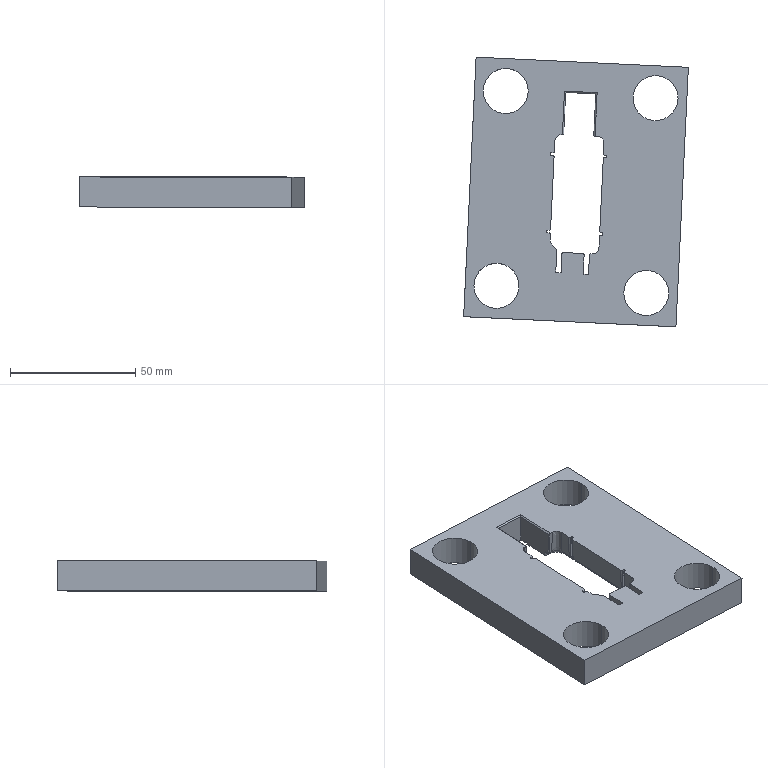Part | STEP file | X77b-01001 | 1 solid | 362 faces | box 89.876 x 107.85 x 12.061 mm | volume 78242 mm3 | cylinder 131 | plane 104 | spline 97 | cone 23 | sphere 6 | torus 1 | commonest cylinder face diameters 1 x83 0.8 x20 4 x9 18 x8 0.332 x5 20 x4